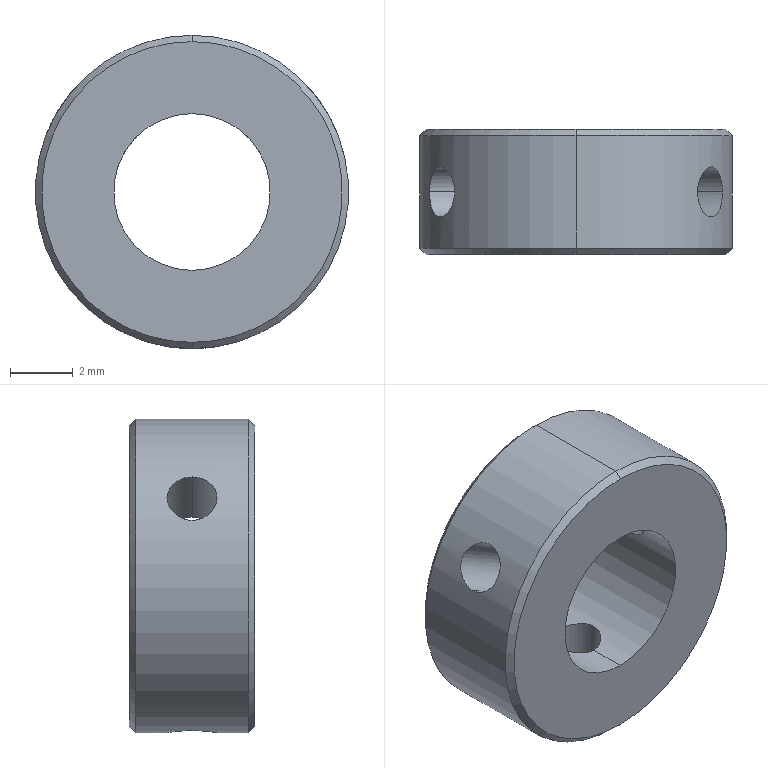Part | NX | features BREP 1 | 1 solid | 16 faces | box 10 x 4 x 10 mm | volume 219.254 mm3 | cylinder 10 | cone 4 | plane 2 | commonest cylinder face diameters 1.6 x6 5 x2 10 x2
STEP:
#1=CARTESIAN_POINT('',(2.451,2.,0.4915));
#2=VERTEX_POINT('',#1);
#3=CARTESIAN_POINT('',(1.651,2.,1.877));
#4=VERTEX_POINT('',#3);
#5=CARTESIAN_POINT('',(2.451,2.,0.4915));
#6=CARTESIAN_POINT('',(2.451,1.802,0.4915));
#7=CARTESIAN_POINT('',(2.423,1.367,0.6755));
#8=CARTESIAN_POINT('',(2.193,1.116,1.265));
#9=CARTESIAN_POINT('',(1.796,1.368,1.762));
#10=CARTESIAN_POINT('',(1.651,1.802,1.877));
#11=CARTESIAN_POINT('',(1.651,2.,1.877));
#12=B_SPLINE_CURVE_WITH_KNOTS('',3,(#5,#6,#7,#8,#9,#10,#11),.UNSPECIFIED.,.F.,.F.,(4,1,1,1,4),(0.,0.25,0.5,0.75,1.),.UNSPECIFIED.);
#13=EDGE_CURVE('',#2,#4,#12,.T.);
#14=ORIENTED_EDGE('',*,*,#13,.T.);
#15=CARTESIAN_POINT('',(3.874,2.,3.161));
#16=VERTEX_POINT('',#15);
#17=CARTESIAN_POINT('',(3.93,2.,3.193));
#18=DIRECTION('',(0.866,0.,0.5));
#19=VECTOR('',#18,1000.);
#20=LINE('',#17,#19);
#21=EDGE_CURVE('',#16,#4,#20,.F.);
#22=ORIENTED_EDGE('',*,*,#21,.F.);
#23=CARTESIAN_POINT('',(4.674,2.,1.775));
#24=VERTEX_POINT('',#23);
#25=CARTESIAN_POINT('',(3.874,2.,3.161));
#26=CARTESIAN_POINT('',(3.874,1.808,3.161));
#27=CARTESIAN_POINT('',(3.989,1.364,3.027));
#28=CARTESIAN_POINT('',(4.344,1.118,2.507));
#29=CARTESIAN_POINT('',(4.616,1.364,1.941));
#30=CARTESIAN_POINT('',(4.674,1.808,1.775));
#31=CARTESIAN_POINT('',(4.674,2.,1.775));
#32=B_SPLINE_CURVE_WITH_KNOTS('',3,(#25,#26,#27,#28,#29,#30,#31),.UNSPECIFIED.,.F.,.F.,(4,1,1,1,4),(0.,0.25,0.5,0.75,1.),.UNSPECIFIED.);
#33=EDGE_CURVE('',#24,#16,#32,.F.);
#34=ORIENTED_EDGE('',*,*,#33,.F.);
#35=CARTESIAN_POINT('',(4.73,2.,1.807));
#36=DIRECTION('',(0.866,0.,0.5));
#37=VECTOR('',#36,1000.);
#38=LINE('',#35,#37);
#39=EDGE_CURVE('',#24,#2,#38,.F.);
#40=ORIENTED_EDGE('',*,*,#39,.T.);
#41=EDGE_LOOP('',(#14,#22,#34,#40));
#42=FACE_BOUND('',#41,.T.);
#43=CARTESIAN_POINT('',(4.33,2.,2.5));
#44=DIRECTION('',(0.866,0.,0.5));
#45=DIRECTION('',(0.5,0.,-0.866));
#46=AXIS2_PLACEMENT_3D('',#43,#44,#45);
#47=CYLINDRICAL_SURFACE('',#46,0.8);
#48=ADVANCED_FACE('',(#42),#47,.F.);
#49=CARTESIAN_POINT('',(-1.651,2.,1.877));
#50=VERTEX_POINT('',#49);
#51=CARTESIAN_POINT('',(-2.451,2.,0.4915));
#52=VERTEX_POINT('',#51);
#53=CARTESIAN_POINT('',(-1.651,2.,1.877));
#54=CARTESIAN_POINT('',(-1.651,1.802,1.877));
#55=CARTESIAN_POINT('',(-1.796,1.367,1.761));
#56=CARTESIAN_POINT('',(-2.192,1.116,1.267));
#57=CARTESIAN_POINT('',(-2.423,1.368,0.6743));
#58=CARTESIAN_POINT('',(-2.451,1.802,0.4915));
#59=CARTESIAN_POINT('',(-2.451,2.,0.4915));
#60=B_SPLINE_CURVE_WITH_KNOTS('',3,(#53,#54,#55,#56,#57,#58,#59),.UNSPECIFIED.,.F.,.F.,(4,1,1,1,4),(0.,0.25,0.5,0.75,1.),.UNSPECIFIED.);
#61=EDGE_CURVE('',#50,#52,#60,.T.);
#62=ORIENTED_EDGE('',*,*,#61,.T.);
#63=CARTESIAN_POINT('',(-4.674,2.,1.775));
#64=VERTEX_POINT('',#63);
#65=CARTESIAN_POINT('',(-4.73,2.,1.807));
#66=DIRECTION('',(-0.866,0.,0.5));
#67=VECTOR('',#66,1000.);
#68=LINE('',#65,#67);
#69=EDGE_CURVE('',#64,#52,#68,.F.);
#70=ORIENTED_EDGE('',*,*,#69,.F.);
#71=CARTESIAN_POINT('',(-3.874,2.,3.161));
#72=VERTEX_POINT('',#71);
#73=CARTESIAN_POINT('',(-4.674,2.,1.775));
#74=CARTESIAN_POINT('',(-4.674,1.808,1.775));
#75=CARTESIAN_POINT('',(-4.616,1.364,1.941));
#76=CARTESIAN_POINT('',(-4.344,1.118,2.509));
#77=CARTESIAN_POINT('',(-3.989,1.364,3.027));
#78=CARTESIAN_POINT('',(-3.874,1.808,3.161));
#79=CARTESIAN_POINT('',(-3.874,2.,3.161));
#80=B_SPLINE_CURVE_WITH_KNOTS('',3,(#73,#74,#75,#76,#77,#78,#79),.UNSPECIFIED.,.F.,.F.,(4,1,1,1,4),(0.,0.25,0.5,0.75,1.),.UNSPECIFIED.);
#81=EDGE_CURVE('',#72,#64,#80,.F.);
#82=ORIENTED_EDGE('',*,*,#81,.F.);
#83=CARTESIAN_POINT('',(-3.93,2.,3.193));
#84=DIRECTION('',(-0.866,0.,0.5));
#85=VECTOR('',#84,1000.);
#86=LINE('',#83,#85);
#87=EDGE_CURVE('',#72,#50,#86,.F.);
#88=ORIENTED_EDGE('',*,*,#87,.T.);
#89=EDGE_LOOP('',(#62,#70,#82,#88));
#90=FACE_BOUND('',#89,.T.);
#91=CARTESIAN_POINT('',(-4.33,2.,2.5));
#92=DIRECTION('',(-0.866,0.,0.5));
#93=DIRECTION('',(0.5,0.,0.866));
#94=AXIS2_PLACEMENT_3D('',#91,#92,#93);
#95=CYLINDRICAL_SURFACE('',#94,0.8);
#96=ADVANCED_FACE('',(#90),#95,.F.);
#97=CARTESIAN_POINT('',(0.,1.2,-2.5));
#98=VERTEX_POINT('',#97);
#99=CARTESIAN_POINT('',(0.8,2.,-2.369));
#100=VERTEX_POINT('',#99);
#101=CARTESIAN_POINT('',(0.,1.2,-2.5));
#102=CARTESIAN_POINT('',(0.1994,1.2,-2.5));
#103=CARTESIAN_POINT('',(0.6317,1.368,-2.436));
#104=CARTESIAN_POINT('',(0.8,1.802,-2.369));
#105=CARTESIAN_POINT('',(0.8,2.,-2.369));
#106=B_SPLINE_CURVE_WITH_KNOTS('',3,(#101,#102,#103,#104,#105),.UNSPECIFIED.,.F.,.F.,(4,1,4),(0.,0.5,1.),.UNSPECIFIED.);
#107=EDGE_CURVE('',#98,#100,#106,.T.);
#108=ORIENTED_EDGE('',*,*,#107,.T.);
#109=CARTESIAN_POINT('',(0.8,2.,-4.936));
#110=VERTEX_POINT('',#109);
#111=CARTESIAN_POINT('',(0.8,2.,-5.));
#112=DIRECTION('',(0.,0.,-1.));
#113=VECTOR('',#112,1000.);
#114=LINE('',#111,#113);
#115=EDGE_CURVE('',#100,#110,#114,.T.);
#116=ORIENTED_EDGE('',*,*,#115,.T.);
#117=CARTESIAN_POINT('',(0.,1.2,-5.));
#118=VERTEX_POINT('',#117);
#119=CARTESIAN_POINT('',(0.8,2.,-4.936));
#120=CARTESIAN_POINT('',(0.8,1.802,-4.936));
#121=CARTESIAN_POINT('',(0.6319,1.367,-4.968));
#122=CARTESIAN_POINT('',(0.1983,1.2,-5.));
#123=CARTESIAN_POINT('',(0.,1.2,-5.));
#124=B_SPLINE_CURVE_WITH_KNOTS('',3,(#119,#120,#121,#122,#123),.UNSPECIFIED.,.F.,.F.,(4,1,4),(0.,0.5,1.),.UNSPECIFIED.);
#125=EDGE_CURVE('',#118,#110,#124,.F.);
#126=ORIENTED_EDGE('',*,*,#125,.F.);
#127=CARTESIAN_POINT('',(-0.8,2.,-4.936));
#128=VERTEX_POINT('',#127);
#129=CARTESIAN_POINT('',(0.,1.2,-5.));
#130=CARTESIAN_POINT('',(-0.1916,1.2,-5.));
#131=CARTESIAN_POINT('',(-0.6354,1.364,-4.968));
#132=CARTESIAN_POINT('',(-0.8,1.809,-4.936));
#133=CARTESIAN_POINT('',(-0.8,2.,-4.936));
#134=B_SPLINE_CURVE_WITH_KNOTS('',3,(#129,#130,#131,#132,#133),.UNSPECIFIED.,.F.,.F.,(4,1,4),(0.,0.5,1.),.UNSPECIFIED.);
#135=EDGE_CURVE('',#128,#118,#134,.F.);
#136=ORIENTED_EDGE('',*,*,#135,.F.);
#137=CARTESIAN_POINT('',(-0.8,2.,-2.369));
#138=VERTEX_POINT('',#137);
#139=CARTESIAN_POINT('',(-0.8,2.,-5.));
#140=DIRECTION('',(0.,0.,-1.));
#141=VECTOR('',#140,1000.);
#142=LINE('',#139,#141);
#143=EDGE_CURVE('',#138,#128,#142,.T.);
#144=ORIENTED_EDGE('',*,*,#143,.F.);
#145=CARTESIAN_POINT('',(-0.8,2.,-2.369));
#146=CARTESIAN_POINT('',(-0.8,1.802,-2.369));
#147=CARTESIAN_POINT('',(-0.631,1.367,-2.436));
#148=CARTESIAN_POINT('',(-0.1994,1.2,-2.5));
#149=CARTESIAN_POINT('',(0.,1.2,-2.5));
#150=B_SPLINE_CURVE_WITH_KNOTS('',3,(#145,#146,#147,#148,#149),.UNSPECIFIED.,.F.,.F.,(4,1,4),(0.,0.5,1.),.UNSPECIFIED.);
#151=EDGE_CURVE('',#138,#98,#150,.T.);
#152=ORIENTED_EDGE('',*,*,#151,.T.);
#153=EDGE_LOOP('',(#108,#116,#126,#136,#144,#152));
#154=FACE_BOUND('',#153,.T.);
#155=CARTESIAN_POINT('',(0.,2.,-5.));
#156=DIRECTION('',(0.,0.,-1.));
#157=DIRECTION('',(-1.,0.,0.));
#158=AXIS2_PLACEMENT_3D('',#155,#156,#157);
#159=CYLINDRICAL_SURFACE('',#158,0.8);
#160=ADVANCED_FACE('',(#154),#159,.F.);
#161=CARTESIAN_POINT('',(0.,4.,4.8));
#162=VERTEX_POINT('',#161);
#163=CARTESIAN_POINT('',(0.,4.,-4.8));
#164=VERTEX_POINT('',#163);
#165=CARTESIAN_POINT('',(0.,4.,0.));
#166=DIRECTION('',(0.,1.,0.));
#167=DIRECTION('',(0.,0.,1.));
#168=AXIS2_PLACEMENT_3D('',#165,#166,#167);
#169=CIRCLE('',#168,4.8);
#170=EDGE_CURVE('',#162,#164,#169,.T.);
#171=ORIENTED_EDGE('',*,*,#170,.F.);
#172=CARTESIAN_POINT('',(0.,3.8,5.));
#173=VERTEX_POINT('',#172);
#174=CARTESIAN_POINT('',(0.,4.,4.8));
#175=DIRECTION('',(0.,-0.7071,0.7071));
#176=VECTOR('',#175,1000.);
#177=LINE('',#174,#176);
#178=EDGE_CURVE('',#162,#173,#177,.T.);
#179=ORIENTED_EDGE('',*,*,#178,.T.);
#180=CARTESIAN_POINT('',(0.,3.8,-5.));
#181=VERTEX_POINT('',#180);
#182=CARTESIAN_POINT('',(0.,3.8,0.));
#183=DIRECTION('',(0.,-1.,0.));
#184=DIRECTION('',(0.,0.,1.));
#185=AXIS2_PLACEMENT_3D('',#182,#183,#184);
#186=CIRCLE('',#185,5.);
#187=EDGE_CURVE('',#181,#173,#186,.T.);
#188=ORIENTED_EDGE('',*,*,#187,.F.);
#189=CARTESIAN_POINT('',(0.,4.,-4.8));
#190=DIRECTION('',(0.,-0.7071,-0.7071));
#191=VECTOR('',#190,1000.);
#192=LINE('',#189,#191);
#193=EDGE_CURVE('',#164,#181,#192,.T.);
#194=ORIENTED_EDGE('',*,*,#193,.F.);
#195=EDGE_LOOP('',(#171,#179,#188,#194));
#196=FACE_BOUND('',#195,.T.);
#197=CARTESIAN_POINT('',(0.,4.,0.));
#198=DIRECTION('',(0.,-1.,0.));
#199=DIRECTION('',(0.,0.,-1.));
#200=AXIS2_PLACEMENT_3D('',#197,#198,#199);
#201=CONICAL_SURFACE('',#200,4.8,0.7854);
#202=ADVANCED_FACE('',(#196),#201,.T.);
#203=CARTESIAN_POINT('',(0.,0.,-4.8));
#204=VERTEX_POINT('',#203);
#205=CARTESIAN_POINT('',(0.,0.,4.8));
#206=VERTEX_POINT('',#205);
#207=CARTESIAN_POINT('',(0.,0.,0.));
#208=DIRECTION('',(0.,-1.,0.));
#209=DIRECTION('',(0.,0.,1.));
#210=AXIS2_PLACEMENT_3D('',#207,#208,#209);
#211=CIRCLE('',#210,4.8);
#212=EDGE_CURVE('',#204,#206,#211,.T.);
#213=ORIENTED_EDGE('',*,*,#212,.F.);
#214=CARTESIAN_POINT('',(0.,0.2,-5.));
#215=VERTEX_POINT('',#214);
#216=CARTESIAN_POINT('',(0.,0.2,-5.));
#217=DIRECTION('',(0.,0.7071,-0.7071));
#218=VECTOR('',#217,1000.);
#219=LINE('',#216,#218);
#220=EDGE_CURVE('',#215,#204,#219,.F.);
#221=ORIENTED_EDGE('',*,*,#220,.F.);
#222=CARTESIAN_POINT('',(0.,0.2,5.));
#223=VERTEX_POINT('',#222);
#224=CARTESIAN_POINT('',(0.,0.2,0.));
#225=DIRECTION('',(0.,1.,0.));
#226=DIRECTION('',(0.,0.,1.));
#227=AXIS2_PLACEMENT_3D('',#224,#225,#226);
#228=CIRCLE('',#227,5.);
#229=EDGE_CURVE('',#223,#215,#228,.T.);
#230=ORIENTED_EDGE('',*,*,#229,.F.);
#231=CARTESIAN_POINT('',(0.,0.2,5.));
#232=DIRECTION('',(0.,0.7071,0.7071));
#233=VECTOR('',#232,1000.);
#234=LINE('',#231,#233);
#235=EDGE_CURVE('',#223,#206,#234,.F.);
#236=ORIENTED_EDGE('',*,*,#235,.T.);
#237=EDGE_LOOP('',(#213,#221,#230,#236));
#238=FACE_BOUND('',#237,.T.);
#239=CARTESIAN_POINT('',(0.,0.2,0.));
#240=DIRECTION('',(0.,1.,0.));
#241=DIRECTION('',(0.,0.,1.));
#242=AXIS2_PLACEMENT_3D('',#239,#240,#241);
#243=CONICAL_SURFACE('',#242,5.,0.7854);
#244=ADVANCED_FACE('',(#238),#243,.T.);
#245=CARTESIAN_POINT('',(0.,4.,-2.5));
#246=VERTEX_POINT('',#245);
#247=CARTESIAN_POINT('',(0.,4.,2.5));
#248=VERTEX_POINT('',#247);
#249=CARTESIAN_POINT('',(0.,4.,0.));
#250=DIRECTION('',(0.,1.,0.));
#251=DIRECTION('',(0.,0.,1.));
#252=AXIS2_PLACEMENT_3D('',#249,#250,#251);
#253=CIRCLE('',#252,2.5);
#254=EDGE_CURVE('',#246,#248,#253,.T.);
#255=ORIENTED_EDGE('',*,*,#254,.T.);
#256=CARTESIAN_POINT('',(0.,0.,2.5));
#257=VERTEX_POINT('',#256);
#258=CARTESIAN_POINT('',(0.,4.,2.5));
#259=DIRECTION('',(0.,-1.,0.));
#260=VECTOR('',#259,1000.);
#261=LINE('',#258,#260);
#262=EDGE_CURVE('',#257,#248,#261,.F.);
#263=ORIENTED_EDGE('',*,*,#262,.F.);
#264=CARTESIAN_POINT('',(0.,0.,-2.5));
#265=VERTEX_POINT('',#264);
#266=CARTESIAN_POINT('',(0.,0.,0.));
#267=DIRECTION('',(0.,1.,0.));
#268=DIRECTION('',(0.,0.,1.));
#269=AXIS2_PLACEMENT_3D('',#266,#267,#268);
#270=CIRCLE('',#269,2.5);
#271=EDGE_CURVE('',#265,#257,#270,.T.);
#272=ORIENTED_EDGE('',*,*,#271,.F.);
#273=CARTESIAN_POINT('',(0.,4.,-2.5));
#274=DIRECTION('',(0.,-1.,0.));
#275=VECTOR('',#274,1000.);
#276=LINE('',#273,#275);
#277=EDGE_CURVE('',#98,#265,#276,.T.);
#278=ORIENTED_EDGE('',*,*,#277,.F.);
#279=ORIENTED_EDGE('',*,*,#151,.F.);
#280=CARTESIAN_POINT('',(0.,2.8,-2.5));
#281=VERTEX_POINT('',#280);
#282=CARTESIAN_POINT('',(-0.8,2.,-2.369));
#283=CARTESIAN_POINT('',(-0.7997,2.425,-2.369));
#284=CARTESIAN_POINT('',(-0.4258,2.8,-2.5));
#285=CARTESIAN_POINT('',(0.,2.8,-2.5));
#286=B_SPLINE_CURVE_WITH_KNOTS('',3,(#282,#283,#284,#285),.UNSPECIFIED.,.F.,.F.,(4,4),(0.,1.),.UNSPECIFIED.);
#287=EDGE_CURVE('',#281,#138,#286,.F.);
#288=ORIENTED_EDGE('',*,*,#287,.F.);
#289=CARTESIAN_POINT('',(0.,4.,-2.5));
#290=DIRECTION('',(0.,-1.,0.));
#291=VECTOR('',#290,1000.);
#292=LINE('',#289,#291);
#293=EDGE_CURVE('',#281,#246,#292,.F.);
#294=ORIENTED_EDGE('',*,*,#293,.T.);
#295=EDGE_LOOP('',(#255,#263,#272,#278,#279,#288,#294));
#296=FACE_BOUND('',#295,.T.);
#297=ORIENTED_EDGE('',*,*,#61,.F.);
#298=CARTESIAN_POINT('',(-1.651,2.,1.877));
#299=CARTESIAN_POINT('',(-1.651,2.426,1.877));
#300=CARTESIAN_POINT('',(-2.279,3.175,1.316));
#301=CARTESIAN_POINT('',(-2.451,2.425,0.4917));
#302=CARTESIAN_POINT('',(-2.451,2.,0.4915));
#303=B_SPLINE_CURVE_WITH_KNOTS('',3,(#298,#299,#300,#301,#302),.UNSPECIFIED.,.F.,.F.,(4,1,4),(0.,0.5,1.),.UNSPECIFIED.);
#304=EDGE_CURVE('',#52,#50,#303,.F.);
#305=ORIENTED_EDGE('',*,*,#304,.F.);
#306=EDGE_LOOP('',(#297,#305));
#307=FACE_BOUND('',#306,.T.);
#308=CARTESIAN_POINT('',(0.,4.,0.));
#309=DIRECTION('',(0.,-1.,0.));
#310=DIRECTION('',(0.,0.,-1.));
#311=AXIS2_PLACEMENT_3D('',#308,#309,#310);
#312=CYLINDRICAL_SURFACE('',#311,2.5);
#313=ADVANCED_FACE('',(#296,#307),#312,.F.);
#314=ORIENTED_EDGE('',*,*,#187,.T.);
#315=CARTESIAN_POINT('',(0.,4.,5.));
#316=DIRECTION('',(0.,-1.,0.));
#317=VECTOR('',#316,1000.);
#318=LINE('',#315,#317);
#319=EDGE_CURVE('',#223,#173,#318,.F.);
#320=ORIENTED_EDGE('',*,*,#319,.F.);
#321=ORIENTED_EDGE('',*,*,#229,.T.);
#322=CARTESIAN_POINT('',(0.,4.,-5.));
#323=DIRECTION('',(0.,-1.,0.));
#324=VECTOR('',#323,1000.);
#325=LINE('',#322,#324);
#326=EDGE_CURVE('',#118,#215,#325,.T.);
#327=ORIENTED_EDGE('',*,*,#326,.F.);
#328=ORIENTED_EDGE('',*,*,#125,.T.);
#329=CARTESIAN_POINT('',(0.,2.8,-5.));
#330=VERTEX_POINT('',#329);
#331=CARTESIAN_POINT('',(0.8,2.,-4.936));
#332=CARTESIAN_POINT('',(0.7979,2.429,-4.936));
#333=CARTESIAN_POINT('',(0.4216,2.8,-5.));
#334=CARTESIAN_POINT('',(0.,2.8,-5.));
#335=B_SPLINE_CURVE_WITH_KNOTS('',3,(#331,#332,#333,#334),.UNSPECIFIED.,.F.,.F.,(4,4),(0.,1.),.UNSPECIFIED.);
#336=EDGE_CURVE('',#110,#330,#335,.T.);
#337=ORIENTED_EDGE('',*,*,#336,.T.);
#338=CARTESIAN_POINT('',(0.,4.,-5.));
#339=DIRECTION('',(0.,-1.,0.));
#340=VECTOR('',#339,1000.);
#341=LINE('',#338,#340);
#342=EDGE_CURVE('',#330,#181,#341,.F.);
#343=ORIENTED_EDGE('',*,*,#342,.T.);
#344=EDGE_LOOP('',(#314,#320,#321,#327,#328,#337,#343));
#345=FACE_BOUND('',#344,.T.);
#346=ORIENTED_EDGE('',*,*,#33,.T.);
#347=CARTESIAN_POINT('',(3.874,2.,3.161));
#348=CARTESIAN_POINT('',(3.875,2.424,3.16));
#349=CARTESIAN_POINT('',(4.385,3.176,2.533));
#350=CARTESIAN_POINT('',(4.674,2.423,1.776));
#351=CARTESIAN_POINT('',(4.674,2.,1.775));
#352=B_SPLINE_CURVE_WITH_KNOTS('',3,(#347,#348,#349,#350,#351),.UNSPECIFIED.,.F.,.F.,(4,1,4),(0.,0.5,1.),.UNSPECIFIED.);
#353=EDGE_CURVE('',#16,#24,#352,.T.);
#354=ORIENTED_EDGE('',*,*,#353,.T.);
#355=EDGE_LOOP('',(#346,#354));
#356=FACE_BOUND('',#355,.T.);
#357=CARTESIAN_POINT('',(0.,4.,0.));
#358=DIRECTION('',(0.,-1.,0.));
#359=DIRECTION('',(0.,0.,-1.));
#360=AXIS2_PLACEMENT_3D('',#357,#358,#359);
#361=CYLINDRICAL_SURFACE('',#360,5.);
#362=ADVANCED_FACE('',(#345,#356),#361,.T.);
#363=CARTESIAN_POINT('',(0.,4.,0.));
#364=DIRECTION('',(0.,1.,0.));
#365=DIRECTION('',(0.,0.,1.));
#366=AXIS2_PLACEMENT_3D('',#363,#364,#365);
#367=CIRCLE('',#366,4.8);
#368=EDGE_CURVE('',#164,#162,#367,.T.);
#369=ORIENTED_EDGE('',*,*,#368,.T.);
#370=ORIENTED_EDGE('',*,*,#170,.T.);
#371=EDGE_LOOP('',(#369,#370));
#372=FACE_BOUND('',#371,.T.);
#373=ORIENTED_EDGE('',*,*,#254,.F.);
#374=CARTESIAN_POINT('',(0.,4.,0.));
#375=DIRECTION('',(0.,1.,0.));
#376=DIRECTION('',(0.,0.,1.));
#377=AXIS2_PLACEMENT_3D('',#374,#375,#376);
#378=CIRCLE('',#377,2.5);
#379=EDGE_CURVE('',#248,#246,#378,.T.);
#380=ORIENTED_EDGE('',*,*,#379,.F.);
#381=EDGE_LOOP('',(#373,#380));
#382=FACE_BOUND('',#381,.T.);
#383=CARTESIAN_POINT('',(0.,4.,0.));
#384=DIRECTION('',(0.,1.,0.));
#385=DIRECTION('',(1.,0.,0.));
#386=AXIS2_PLACEMENT_3D('',#383,#384,#385);
#387=PLANE('',#386);
#388=ADVANCED_FACE('',(#372,#382),#387,.T.);
#389=CARTESIAN_POINT('',(0.,0.,0.));
#390=DIRECTION('',(0.,-1.,0.));
#391=DIRECTION('',(0.,0.,1.));
#392=AXIS2_PLACEMENT_3D('',#389,#390,#391);
#393=CIRCLE('',#392,4.8);
#394=EDGE_CURVE('',#206,#204,#393,.T.);
#395=ORIENTED_EDGE('',*,*,#394,.T.);
#396=ORIENTED_EDGE('',*,*,#212,.T.);
#397=EDGE_LOOP('',(#395,#396));
#398=FACE_BOUND('',#397,.T.);
#399=ORIENTED_EDGE('',*,*,#271,.T.);
#400=CARTESIAN_POINT('',(0.,0.,0.));
#401=DIRECTION('',(0.,1.,0.));
#402=DIRECTION('',(0.,0.,1.));
#403=AXIS2_PLACEMENT_3D('',#400,#401,#402);
#404=CIRCLE('',#403,2.5);
#405=EDGE_CURVE('',#257,#265,#404,.T.);
#406=ORIENTED_EDGE('',*,*,#405,.T.);
#407=EDGE_LOOP('',(#399,#406));
#408=FACE_BOUND('',#407,.T.);
#409=CARTESIAN_POINT('',(0.,0.,0.));
#410=DIRECTION('',(0.,1.,0.));
#411=DIRECTION('',(1.,0.,0.));
#412=AXIS2_PLACEMENT_3D('',#409,#410,#411);
#413=PLANE('',#412);
#414=ADVANCED_FACE('',(#398,#408),#413,.F.);
#415=ORIENTED_EDGE('',*,*,#319,.T.);
#416=CARTESIAN_POINT('',(0.,3.8,0.));
#417=DIRECTION('',(0.,-1.,0.));
#418=DIRECTION('',(0.,0.,1.));
#419=AXIS2_PLACEMENT_3D('',#416,#417,#418);
#420=CIRCLE('',#419,5.);
#421=EDGE_CURVE('',#173,#181,#420,.T.);
#422=ORIENTED_EDGE('',*,*,#421,.T.);
#423=ORIENTED_EDGE('',*,*,#342,.F.);
#424=CARTESIAN_POINT('',(0.,2.8,-5.));
#425=CARTESIAN_POINT('',(-0.4249,2.8,-5.));
#426=CARTESIAN_POINT('',(-0.7994,2.425,-4.936));
#427=CARTESIAN_POINT('',(-0.8,2.,-4.936));
#428=B_SPLINE_CURVE_WITH_KNOTS('',3,(#424,#425,#426,#427),.UNSPECIFIED.,.F.,.F.,(4,4),(0.,1.),.UNSPECIFIED.);
#429=EDGE_CURVE('',#330,#128,#428,.T.);
#430=ORIENTED_EDGE('',*,*,#429,.T.);
#431=ORIENTED_EDGE('',*,*,#135,.T.);
#432=ORIENTED_EDGE('',*,*,#326,.T.);
#433=CARTESIAN_POINT('',(0.,0.2,0.));
#434=DIRECTION('',(0.,1.,0.));
#435=DIRECTION('',(0.,0.,1.));
#436=AXIS2_PLACEMENT_3D('',#433,#434,#435);
#437=CIRCLE('',#436,5.);
#438=EDGE_CURVE('',#215,#223,#437,.T.);
#439=ORIENTED_EDGE('',*,*,#438,.T.);
#440=EDGE_LOOP('',(#415,#422,#423,#430,#431,#432,#439));
#441=FACE_BOUND('',#440,.T.);
#442=ORIENTED_EDGE('',*,*,#81,.T.);
#443=CARTESIAN_POINT('',(-4.674,2.,1.775));
#444=CARTESIAN_POINT('',(-4.674,2.424,1.776));
#445=CARTESIAN_POINT('',(-4.386,3.176,2.531));
#446=CARTESIAN_POINT('',(-3.875,2.423,3.16));
#447=CARTESIAN_POINT('',(-3.874,2.,3.161));
#448=B_SPLINE_CURVE_WITH_KNOTS('',3,(#443,#444,#445,#446,#447),.UNSPECIFIED.,.F.,.F.,(4,1,4),(0.,0.5,1.),.UNSPECIFIED.);
#449=EDGE_CURVE('',#64,#72,#448,.T.);
#450=ORIENTED_EDGE('',*,*,#449,.T.);
#451=EDGE_LOOP('',(#442,#450));
#452=FACE_BOUND('',#451,.T.);
#453=CARTESIAN_POINT('',(0.,4.,0.));
#454=DIRECTION('',(0.,-1.,0.));
#455=DIRECTION('',(0.,0.,-1.));
#456=AXIS2_PLACEMENT_3D('',#453,#454,#455);
#457=CYLINDRICAL_SURFACE('',#456,5.);
#458=ADVANCED_FACE('',(#441,#452),#457,.T.);
#459=ORIENTED_EDGE('',*,*,#262,.T.);
#460=ORIENTED_EDGE('',*,*,#379,.T.);
#461=ORIENTED_EDGE('',*,*,#293,.F.);
#462=CARTESIAN_POINT('',(0.,2.8,-2.5));
#463=CARTESIAN_POINT('',(0.4257,2.8,-2.5));
#464=CARTESIAN_POINT('',(0.7997,2.425,-2.369));
#465=CARTESIAN_POINT('',(0.8,2.,-2.369));
#466=B_SPLINE_CURVE_WITH_KNOTS('',3,(#462,#463,#464,#465),.UNSPECIFIED.,.F.,.F.,(4,4),(0.,1.),.UNSPECIFIED.);
#467=EDGE_CURVE('',#100,#281,#466,.F.);
#468=ORIENTED_EDGE('',*,*,#467,.F.);
#469=ORIENTED_EDGE('',*,*,#107,.F.);
#470=ORIENTED_EDGE('',*,*,#277,.T.);
#471=ORIENTED_EDGE('',*,*,#405,.F.);
#472=EDGE_LOOP('',(#459,#460,#461,#468,#469,#470,#471));
#473=FACE_BOUND('',#472,.T.);
#474=ORIENTED_EDGE('',*,*,#13,.F.);
#475=CARTESIAN_POINT('',(2.451,2.,0.4915));
#476=CARTESIAN_POINT('',(2.451,2.426,0.4917));
#477=CARTESIAN_POINT('',(2.279,3.175,1.316));
#478=CARTESIAN_POINT('',(1.651,2.425,1.877));
#479=CARTESIAN_POINT('',(1.651,2.,1.877));
#480=B_SPLINE_CURVE_WITH_KNOTS('',3,(#475,#476,#477,#478,#479),.UNSPECIFIED.,.F.,.F.,(4,1,4),(0.,0.5,1.),.UNSPECIFIED.);
#481=EDGE_CURVE('',#4,#2,#480,.F.);
#482=ORIENTED_EDGE('',*,*,#481,.F.);
#483=EDGE_LOOP('',(#474,#482));
#484=FACE_BOUND('',#483,.T.);
#485=CARTESIAN_POINT('',(0.,4.,0.));
#486=DIRECTION('',(0.,-1.,0.));
#487=DIRECTION('',(0.,0.,-1.));
#488=AXIS2_PLACEMENT_3D('',#485,#486,#487);
#489=CYLINDRICAL_SURFACE('',#488,2.5);
#490=ADVANCED_FACE('',(#473,#484),#489,.F.);
#491=ORIENTED_EDGE('',*,*,#220,.T.);
#492=ORIENTED_EDGE('',*,*,#394,.F.);
#493=ORIENTED_EDGE('',*,*,#235,.F.);
#494=ORIENTED_EDGE('',*,*,#438,.F.);
#495=EDGE_LOOP('',(#491,#492,#493,#494));
#496=FACE_BOUND('',#495,.T.);
#497=CARTESIAN_POINT('',(0.,0.2,0.));
#498=DIRECTION('',(0.,1.,0.));
#499=DIRECTION('',(0.,0.,1.));
#500=AXIS2_PLACEMENT_3D('',#497,#498,#499);
#501=CONICAL_SURFACE('',#500,5.,0.7854);
#502=ADVANCED_FACE('',(#496),#501,.T.);
#503=ORIENTED_EDGE('',*,*,#178,.F.);
#504=ORIENTED_EDGE('',*,*,#368,.F.);
#505=ORIENTED_EDGE('',*,*,#193,.T.);
#506=ORIENTED_EDGE('',*,*,#421,.F.);
#507=EDGE_LOOP('',(#503,#504,#505,#506));
#508=FACE_BOUND('',#507,.T.);
#509=CARTESIAN_POINT('',(0.,4.,0.));
#510=DIRECTION('',(0.,-1.,0.));
#511=DIRECTION('',(0.,0.,-1.));
#512=AXIS2_PLACEMENT_3D('',#509,#510,#511);
#513=CONICAL_SURFACE('',#512,4.8,0.7854);
#514=ADVANCED_FACE('',(#508),#513,.T.);
#515=ORIENTED_EDGE('',*,*,#115,.F.);
#516=ORIENTED_EDGE('',*,*,#467,.T.);
#517=ORIENTED_EDGE('',*,*,#287,.T.);
#518=ORIENTED_EDGE('',*,*,#143,.T.);
#519=ORIENTED_EDGE('',*,*,#429,.F.);
#520=ORIENTED_EDGE('',*,*,#336,.F.);
#521=EDGE_LOOP('',(#515,#516,#517,#518,#519,#520));
#522=FACE_BOUND('',#521,.T.);
#523=CARTESIAN_POINT('',(0.,2.,-5.));
#524=DIRECTION('',(0.,0.,-1.));
#525=DIRECTION('',(-1.,0.,0.));
#526=AXIS2_PLACEMENT_3D('',#523,#524,#525);
#527=CYLINDRICAL_SURFACE('',#526,0.8);
#528=ADVANCED_FACE('',(#522),#527,.F.);
#529=ORIENTED_EDGE('',*,*,#69,.T.);
#530=ORIENTED_EDGE('',*,*,#304,.T.);
#531=ORIENTED_EDGE('',*,*,#87,.F.);
#532=ORIENTED_EDGE('',*,*,#449,.F.);
#533=EDGE_LOOP('',(#529,#530,#531,#532));
#534=FACE_BOUND('',#533,.T.);
#535=CARTESIAN_POINT('',(-4.33,2.,2.5));
#536=DIRECTION('',(-0.866,0.,0.5));
#537=DIRECTION('',(0.5,0.,0.866));
#538=AXIS2_PLACEMENT_3D('',#535,#536,#537);
#539=CYLINDRICAL_SURFACE('',#538,0.8);
#540=ADVANCED_FACE('',(#534),#539,.F.);
#541=ORIENTED_EDGE('',*,*,#21,.T.);
#542=ORIENTED_EDGE('',*,*,#481,.T.);
#543=ORIENTED_EDGE('',*,*,#39,.F.);
#544=ORIENTED_EDGE('',*,*,#353,.F.);
#545=EDGE_LOOP('',(#541,#542,#543,#544));
#546=FACE_BOUND('',#545,.T.);
#547=CARTESIAN_POINT('',(4.33,2.,2.5));
#548=DIRECTION('',(0.866,0.,0.5));
#549=DIRECTION('',(0.5,0.,-0.866));
#550=AXIS2_PLACEMENT_3D('',#547,#548,#549);
#551=CYLINDRICAL_SURFACE('',#550,0.8);
#552=ADVANCED_FACE('',(#546),#551,.F.);
#553=CLOSED_SHELL('',(#48,#96,#160,#202,#244,#313,#362,#388,#414,#458,#490,#502,#514,#528,#540,#552));
#554=MANIFOLD_SOLID_BREP('',#553);
#555=(LENGTH_UNIT()NAMED_UNIT(*)SI_UNIT(.MILLI.,.METRE.));
#556=UNCERTAINTY_MEASURE_WITH_UNIT(LENGTH_MEASURE(0.0508),#555,'','');
#557=(NAMED_UNIT(*)PLANE_ANGLE_UNIT()SI_UNIT($,.RADIAN.));
#558=(NAMED_UNIT(*)SI_UNIT($,.STERADIAN.)SOLID_ANGLE_UNIT());
#559=(GEOMETRIC_REPRESENTATION_CONTEXT(3)GLOBAL_UNCERTAINTY_ASSIGNED_CONTEXT((#556))GLOBAL_UNIT_ASSIGNED_CONTEXT((#555,#557,#558))REPRESENTATION_CONTEXT('',''));
#560=ADVANCED_BREP_SHAPE_REPRESENTATION('',(#554),#559);